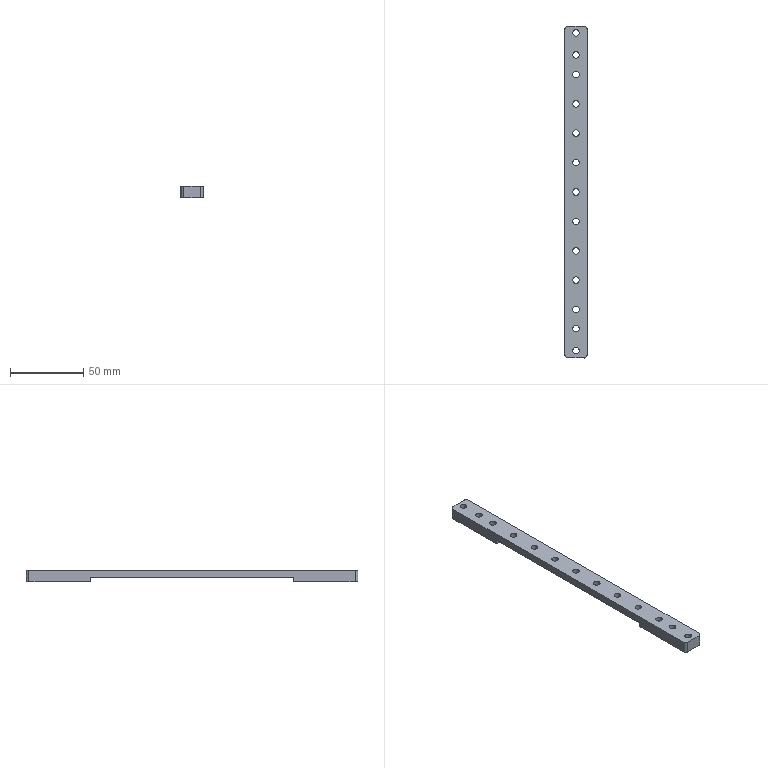Part | STEP file | SOLID | 1 solid | 27 faces | box 15 x 226 x 8 mm | volume 19553 mm3 | cylinder 17 | plane 10 | commonest cylinder face diameters 4.5 x13 4 x4